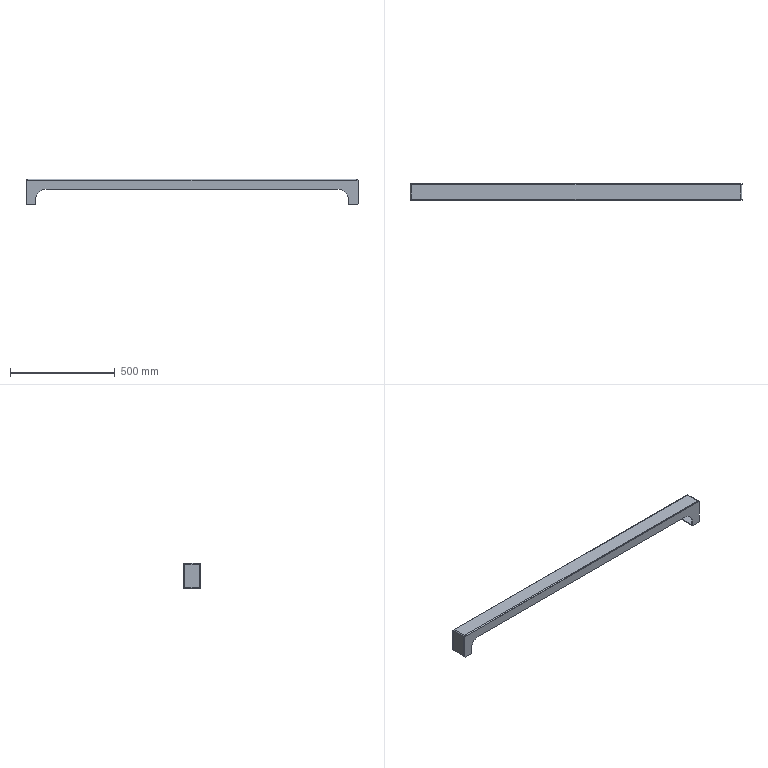Part | STEP file | SYL_0392D6J1SYL0380DJ10-1531669 | 1 solid | 82 faces | box 1585 x 77.2 x 123.6 mm | volume 1073180 mm3 | plane 66 | cylinder 16 | commonest cylinder face diameters 2 x6 9.2 x6 100 x4